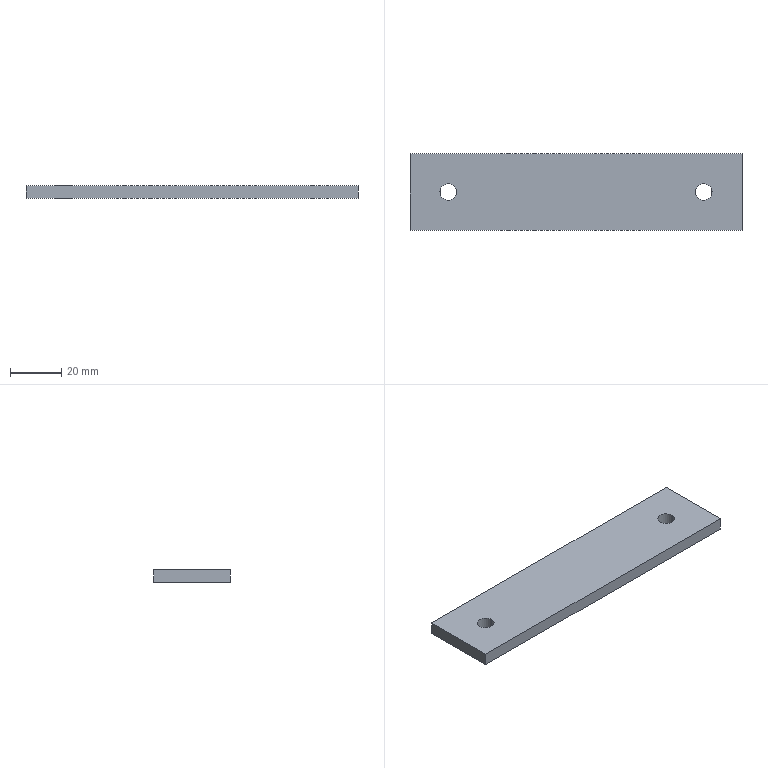Part | SolidWorks | features MirrorStock 1 | 1 solid | 10 faces | box 130 x 30 x 5 mm | volume 19158 mm3 | plane 6 | cylinder 4 | commonest cylinder face diameters 6.6 x4
STEP:
#1=CARTESIAN_POINT('',(53.3,0.,-5.));
#2=VERTEX_POINT('',#1);
#3=CARTESIAN_POINT('',(46.7,0.,-5.));
#4=VERTEX_POINT('',#3);
#5=CARTESIAN_POINT('',(50.,0.,-5.));
#6=DIRECTION('',(0.,0.,1.));
#7=DIRECTION('',(1.,0.,0.));
#8=AXIS2_PLACEMENT_3D('',#5,#6,#7);
#9=CIRCLE('',#8,3.3);
#10=EDGE_CURVE('',#2,#4,#9,.T.);
#11=ORIENTED_EDGE('',*,*,#10,.F.);
#12=CARTESIAN_POINT('',(53.3,0.,0.));
#13=VERTEX_POINT('',#12);
#14=CARTESIAN_POINT('',(53.3,0.,-5.));
#15=DIRECTION('',(0.,0.,1.));
#16=VECTOR('',#15,1000.);
#17=LINE('',#14,#16);
#18=EDGE_CURVE('',#2,#13,#17,.T.);
#19=ORIENTED_EDGE('',*,*,#18,.T.);
#20=CARTESIAN_POINT('',(46.7,0.,0.));
#21=VERTEX_POINT('',#20);
#22=CARTESIAN_POINT('',(50.,0.,0.));
#23=DIRECTION('',(0.,0.,1.));
#24=DIRECTION('',(1.,0.,0.));
#25=AXIS2_PLACEMENT_3D('',#22,#23,#24);
#26=CIRCLE('',#25,3.3);
#27=EDGE_CURVE('',#13,#21,#26,.T.);
#28=ORIENTED_EDGE('',*,*,#27,.T.);
#29=CARTESIAN_POINT('',(46.7,0.,-5.));
#30=DIRECTION('',(0.,0.,1.));
#31=VECTOR('',#30,1000.);
#32=LINE('',#29,#31);
#33=EDGE_CURVE('',#4,#21,#32,.T.);
#34=ORIENTED_EDGE('',*,*,#33,.F.);
#35=EDGE_LOOP('',(#11,#19,#28,#34));
#36=FACE_OUTER_BOUND('',#35,.T.);
#37=CARTESIAN_POINT('',(50.,0.,-5.));
#38=DIRECTION('',(0.,0.,1.));
#39=DIRECTION('',(-1.,0.,0.));
#40=AXIS2_PLACEMENT_3D('',#37,#38,#39);
#41=CYLINDRICAL_SURFACE('',#40,3.3);
#42=ADVANCED_FACE('',(#36),#41,.F.);
#43=CARTESIAN_POINT('',(-46.7,0.,-5.));
#44=VERTEX_POINT('',#43);
#45=CARTESIAN_POINT('',(-53.3,0.,-5.));
#46=VERTEX_POINT('',#45);
#47=CARTESIAN_POINT('',(-50.,0.,-5.));
#48=DIRECTION('',(0.,0.,1.));
#49=DIRECTION('',(1.,0.,0.));
#50=AXIS2_PLACEMENT_3D('',#47,#48,#49);
#51=CIRCLE('',#50,3.3);
#52=EDGE_CURVE('',#44,#46,#51,.T.);
#53=ORIENTED_EDGE('',*,*,#52,.F.);
#54=CARTESIAN_POINT('',(-46.7,0.,0.));
#55=VERTEX_POINT('',#54);
#56=CARTESIAN_POINT('',(-46.7,0.,-5.));
#57=DIRECTION('',(0.,0.,1.));
#58=VECTOR('',#57,1000.);
#59=LINE('',#56,#58);
#60=EDGE_CURVE('',#44,#55,#59,.T.);
#61=ORIENTED_EDGE('',*,*,#60,.T.);
#62=CARTESIAN_POINT('',(-53.3,0.,0.));
#63=VERTEX_POINT('',#62);
#64=CARTESIAN_POINT('',(-50.,0.,0.));
#65=DIRECTION('',(0.,0.,1.));
#66=DIRECTION('',(1.,0.,0.));
#67=AXIS2_PLACEMENT_3D('',#64,#65,#66);
#68=CIRCLE('',#67,3.3);
#69=EDGE_CURVE('',#55,#63,#68,.T.);
#70=ORIENTED_EDGE('',*,*,#69,.T.);
#71=CARTESIAN_POINT('',(-53.3,0.,-5.));
#72=DIRECTION('',(0.,0.,1.));
#73=VECTOR('',#72,1000.);
#74=LINE('',#71,#73);
#75=EDGE_CURVE('',#46,#63,#74,.T.);
#76=ORIENTED_EDGE('',*,*,#75,.F.);
#77=EDGE_LOOP('',(#53,#61,#70,#76));
#78=FACE_OUTER_BOUND('',#77,.T.);
#79=CARTESIAN_POINT('',(-50.,0.,-5.));
#80=DIRECTION('',(0.,0.,1.));
#81=DIRECTION('',(-1.,0.,0.));
#82=AXIS2_PLACEMENT_3D('',#79,#80,#81);
#83=CYLINDRICAL_SURFACE('',#82,3.3);
#84=ADVANCED_FACE('',(#78),#83,.F.);
#85=CARTESIAN_POINT('',(-50.,0.,-5.));
#86=DIRECTION('',(0.,0.,1.));
#87=DIRECTION('',(1.,0.,0.));
#88=AXIS2_PLACEMENT_3D('',#85,#86,#87);
#89=CIRCLE('',#88,3.3);
#90=EDGE_CURVE('',#46,#44,#89,.T.);
#91=ORIENTED_EDGE('',*,*,#90,.T.);
#92=ORIENTED_EDGE('',*,*,#52,.T.);
#93=EDGE_LOOP('',(#91,#92));
#94=FACE_BOUND('',#93,.T.);
#95=CARTESIAN_POINT('',(-65.,15.,-5.));
#96=VERTEX_POINT('',#95);
#97=CARTESIAN_POINT('',(-65.,-15.,-5.));
#98=VERTEX_POINT('',#97);
#99=CARTESIAN_POINT('',(-65.,-15.,-5.));
#100=DIRECTION('',(0.,-1.,0.));
#101=VECTOR('',#100,1000.);
#102=LINE('',#99,#101);
#103=EDGE_CURVE('',#96,#98,#102,.T.);
#104=ORIENTED_EDGE('',*,*,#103,.F.);
#105=CARTESIAN_POINT('',(65.,15.,-5.));
#106=VERTEX_POINT('',#105);
#107=CARTESIAN_POINT('',(65.,15.,-5.));
#108=DIRECTION('',(-1.,0.,0.));
#109=VECTOR('',#108,1000.);
#110=LINE('',#107,#109);
#111=EDGE_CURVE('',#106,#96,#110,.T.);
#112=ORIENTED_EDGE('',*,*,#111,.F.);
#113=CARTESIAN_POINT('',(65.,-15.,-5.));
#114=VERTEX_POINT('',#113);
#115=CARTESIAN_POINT('',(65.,-15.,-5.));
#116=DIRECTION('',(0.,1.,0.));
#117=VECTOR('',#116,1000.);
#118=LINE('',#115,#117);
#119=EDGE_CURVE('',#114,#106,#118,.T.);
#120=ORIENTED_EDGE('',*,*,#119,.F.);
#121=CARTESIAN_POINT('',(65.,-15.,-5.));
#122=DIRECTION('',(1.,0.,0.));
#123=VECTOR('',#122,1000.);
#124=LINE('',#121,#123);
#125=EDGE_CURVE('',#98,#114,#124,.T.);
#126=ORIENTED_EDGE('',*,*,#125,.F.);
#127=EDGE_LOOP('',(#104,#112,#120,#126));
#128=FACE_OUTER_BOUND('',#127,.T.);
#129=CARTESIAN_POINT('',(50.,0.,-5.));
#130=DIRECTION('',(0.,0.,1.));
#131=DIRECTION('',(1.,0.,0.));
#132=AXIS2_PLACEMENT_3D('',#129,#130,#131);
#133=CIRCLE('',#132,3.3);
#134=EDGE_CURVE('',#4,#2,#133,.T.);
#135=ORIENTED_EDGE('',*,*,#134,.T.);
#136=ORIENTED_EDGE('',*,*,#10,.T.);
#137=EDGE_LOOP('',(#135,#136));
#138=FACE_BOUND('',#137,.T.);
#139=CARTESIAN_POINT('',(0.,0.,-5.));
#140=DIRECTION('',(0.,0.,-1.));
#141=DIRECTION('',(1.,0.,0.));
#142=AXIS2_PLACEMENT_3D('',#139,#140,#141);
#143=PLANE('',#142);
#144=ADVANCED_FACE('',(#94,#128,#138),#143,.T.);
#145=CARTESIAN_POINT('',(-65.,15.,0.));
#146=VERTEX_POINT('',#145);
#147=CARTESIAN_POINT('',(-65.,-15.,0.));
#148=VERTEX_POINT('',#147);
#149=CARTESIAN_POINT('',(-65.,-15.,0.));
#150=DIRECTION('',(0.,-1.,0.));
#151=VECTOR('',#150,1000.);
#152=LINE('',#149,#151);
#153=EDGE_CURVE('',#146,#148,#152,.T.);
#154=ORIENTED_EDGE('',*,*,#153,.T.);
#155=CARTESIAN_POINT('',(65.,-15.,0.));
#156=VERTEX_POINT('',#155);
#157=CARTESIAN_POINT('',(65.,-15.,0.));
#158=DIRECTION('',(1.,0.,0.));
#159=VECTOR('',#158,1000.);
#160=LINE('',#157,#159);
#161=EDGE_CURVE('',#148,#156,#160,.T.);
#162=ORIENTED_EDGE('',*,*,#161,.T.);
#163=CARTESIAN_POINT('',(65.,15.,0.));
#164=VERTEX_POINT('',#163);
#165=CARTESIAN_POINT('',(65.,-15.,0.));
#166=DIRECTION('',(0.,1.,0.));
#167=VECTOR('',#166,1000.);
#168=LINE('',#165,#167);
#169=EDGE_CURVE('',#156,#164,#168,.T.);
#170=ORIENTED_EDGE('',*,*,#169,.T.);
#171=CARTESIAN_POINT('',(65.,15.,0.));
#172=DIRECTION('',(-1.,0.,0.));
#173=VECTOR('',#172,1000.);
#174=LINE('',#171,#173);
#175=EDGE_CURVE('',#164,#146,#174,.T.);
#176=ORIENTED_EDGE('',*,*,#175,.T.);
#177=EDGE_LOOP('',(#154,#162,#170,#176));
#178=FACE_OUTER_BOUND('',#177,.T.);
#179=CARTESIAN_POINT('',(-50.,0.,0.));
#180=DIRECTION('',(0.,0.,1.));
#181=DIRECTION('',(1.,0.,0.));
#182=AXIS2_PLACEMENT_3D('',#179,#180,#181);
#183=CIRCLE('',#182,3.3);
#184=EDGE_CURVE('',#63,#55,#183,.T.);
#185=ORIENTED_EDGE('',*,*,#184,.F.);
#186=ORIENTED_EDGE('',*,*,#69,.F.);
#187=EDGE_LOOP('',(#185,#186));
#188=FACE_BOUND('',#187,.T.);
#189=CARTESIAN_POINT('',(50.,0.,0.));
#190=DIRECTION('',(0.,0.,1.));
#191=DIRECTION('',(1.,0.,0.));
#192=AXIS2_PLACEMENT_3D('',#189,#190,#191);
#193=CIRCLE('',#192,3.3);
#194=EDGE_CURVE('',#21,#13,#193,.T.);
#195=ORIENTED_EDGE('',*,*,#194,.F.);
#196=ORIENTED_EDGE('',*,*,#27,.F.);
#197=EDGE_LOOP('',(#195,#196));
#198=FACE_BOUND('',#197,.T.);
#199=CARTESIAN_POINT('',(0.,0.,0.));
#200=DIRECTION('',(0.,0.,-1.));
#201=DIRECTION('',(1.,0.,0.));
#202=AXIS2_PLACEMENT_3D('',#199,#200,#201);
#203=PLANE('',#202);
#204=ADVANCED_FACE('',(#178,#188,#198),#203,.F.);
#205=ORIENTED_EDGE('',*,*,#153,.F.);
#206=CARTESIAN_POINT('',(-65.,15.,-5.));
#207=DIRECTION('',(0.,0.,1.));
#208=VECTOR('',#207,1000.);
#209=LINE('',#206,#208);
#210=EDGE_CURVE('',#96,#146,#209,.T.);
#211=ORIENTED_EDGE('',*,*,#210,.F.);
#212=ORIENTED_EDGE('',*,*,#103,.T.);
#213=CARTESIAN_POINT('',(-65.,-15.,-5.));
#214=DIRECTION('',(0.,0.,1.));
#215=VECTOR('',#214,1000.);
#216=LINE('',#213,#215);
#217=EDGE_CURVE('',#98,#148,#216,.T.);
#218=ORIENTED_EDGE('',*,*,#217,.T.);
#219=EDGE_LOOP('',(#205,#211,#212,#218));
#220=FACE_OUTER_BOUND('',#219,.T.);
#221=CARTESIAN_POINT('',(-65.,-15.,-5.));
#222=DIRECTION('',(1.,0.,0.));
#223=DIRECTION('',(0.,0.,1.));
#224=AXIS2_PLACEMENT_3D('',#221,#222,#223);
#225=PLANE('',#224);
#226=ADVANCED_FACE('',(#220),#225,.F.);
#227=ORIENTED_EDGE('',*,*,#161,.F.);
#228=ORIENTED_EDGE('',*,*,#217,.F.);
#229=ORIENTED_EDGE('',*,*,#125,.T.);
#230=CARTESIAN_POINT('',(65.,-15.,-5.));
#231=DIRECTION('',(0.,0.,1.));
#232=VECTOR('',#231,1000.);
#233=LINE('',#230,#232);
#234=EDGE_CURVE('',#114,#156,#233,.T.);
#235=ORIENTED_EDGE('',*,*,#234,.T.);
#236=EDGE_LOOP('',(#227,#228,#229,#235));
#237=FACE_OUTER_BOUND('',#236,.T.);
#238=CARTESIAN_POINT('',(65.,-15.,-5.));
#239=DIRECTION('',(0.,1.,0.));
#240=DIRECTION('',(-1.,0.,0.));
#241=AXIS2_PLACEMENT_3D('',#238,#239,#240);
#242=PLANE('',#241);
#243=ADVANCED_FACE('',(#237),#242,.F.);
#244=ORIENTED_EDGE('',*,*,#169,.F.);
#245=ORIENTED_EDGE('',*,*,#234,.F.);
#246=ORIENTED_EDGE('',*,*,#119,.T.);
#247=CARTESIAN_POINT('',(65.,15.,-5.));
#248=DIRECTION('',(0.,0.,1.));
#249=VECTOR('',#248,1000.);
#250=LINE('',#247,#249);
#251=EDGE_CURVE('',#106,#164,#250,.T.);
#252=ORIENTED_EDGE('',*,*,#251,.T.);
#253=EDGE_LOOP('',(#244,#245,#246,#252));
#254=FACE_OUTER_BOUND('',#253,.T.);
#255=CARTESIAN_POINT('',(65.,-15.,-5.));
#256=DIRECTION('',(-1.,0.,0.));
#257=DIRECTION('',(0.,0.,-1.));
#258=AXIS2_PLACEMENT_3D('',#255,#256,#257);
#259=PLANE('',#258);
#260=ADVANCED_FACE('',(#254),#259,.F.);
#261=ORIENTED_EDGE('',*,*,#175,.F.);
#262=ORIENTED_EDGE('',*,*,#251,.F.);
#263=ORIENTED_EDGE('',*,*,#111,.T.);
#264=ORIENTED_EDGE('',*,*,#210,.T.);
#265=EDGE_LOOP('',(#261,#262,#263,#264));
#266=FACE_OUTER_BOUND('',#265,.T.);
#267=CARTESIAN_POINT('',(65.,15.,-5.));
#268=DIRECTION('',(0.,-1.,0.));
#269=DIRECTION('',(1.,0.,0.));
#270=AXIS2_PLACEMENT_3D('',#267,#268,#269);
#271=PLANE('',#270);
#272=ADVANCED_FACE('',(#266),#271,.F.);
#273=ORIENTED_EDGE('',*,*,#60,.F.);
#274=ORIENTED_EDGE('',*,*,#90,.F.);
#275=ORIENTED_EDGE('',*,*,#75,.T.);
#276=ORIENTED_EDGE('',*,*,#184,.T.);
#277=EDGE_LOOP('',(#273,#274,#275,#276));
#278=FACE_OUTER_BOUND('',#277,.T.);
#279=CARTESIAN_POINT('',(-50.,0.,-5.));
#280=DIRECTION('',(0.,0.,1.));
#281=DIRECTION('',(-1.,0.,0.));
#282=AXIS2_PLACEMENT_3D('',#279,#280,#281);
#283=CYLINDRICAL_SURFACE('',#282,3.3);
#284=ADVANCED_FACE('',(#278),#283,.F.);
#285=ORIENTED_EDGE('',*,*,#18,.F.);
#286=ORIENTED_EDGE('',*,*,#134,.F.);
#287=ORIENTED_EDGE('',*,*,#33,.T.);
#288=ORIENTED_EDGE('',*,*,#194,.T.);
#289=EDGE_LOOP('',(#285,#286,#287,#288));
#290=FACE_OUTER_BOUND('',#289,.T.);
#291=CARTESIAN_POINT('',(50.,0.,-5.));
#292=DIRECTION('',(0.,0.,1.));
#293=DIRECTION('',(-1.,0.,0.));
#294=AXIS2_PLACEMENT_3D('',#291,#292,#293);
#295=CYLINDRICAL_SURFACE('',#294,3.3);
#296=ADVANCED_FACE('',(#290),#295,.F.);
#297=CLOSED_SHELL('',(#42,#84,#144,#204,#226,#243,#260,#272,#284,#296));
#298=MANIFOLD_SOLID_BREP('',#297);
#299=CARTESIAN_POINT('',(0.,0.,0.));
#300=DIRECTION('',(0.,0.,1.));
#301=DIRECTION('',(1.,0.,0.));
#302=AXIS2_PLACEMENT_3D('',#299,#300,#301);
#303=(LENGTH_UNIT()NAMED_UNIT(*)SI_UNIT(.MILLI.,.METRE.));
#304=UNCERTAINTY_MEASURE_WITH_UNIT(LENGTH_MEASURE(0.00001),#303,'','');
#305=(NAMED_UNIT(*)PLANE_ANGLE_UNIT()SI_UNIT($,.RADIAN.));
#306=(NAMED_UNIT(*)SI_UNIT($,.STERADIAN.)SOLID_ANGLE_UNIT());
#307=(GEOMETRIC_REPRESENTATION_CONTEXT(3)GLOBAL_UNCERTAINTY_ASSIGNED_CONTEXT((#304))GLOBAL_UNIT_ASSIGNED_CONTEXT((#303,#305,#306))REPRESENTATION_CONTEXT('',''));
#308=ADVANCED_BREP_SHAPE_REPRESENTATION('',(#298,#302),#307);